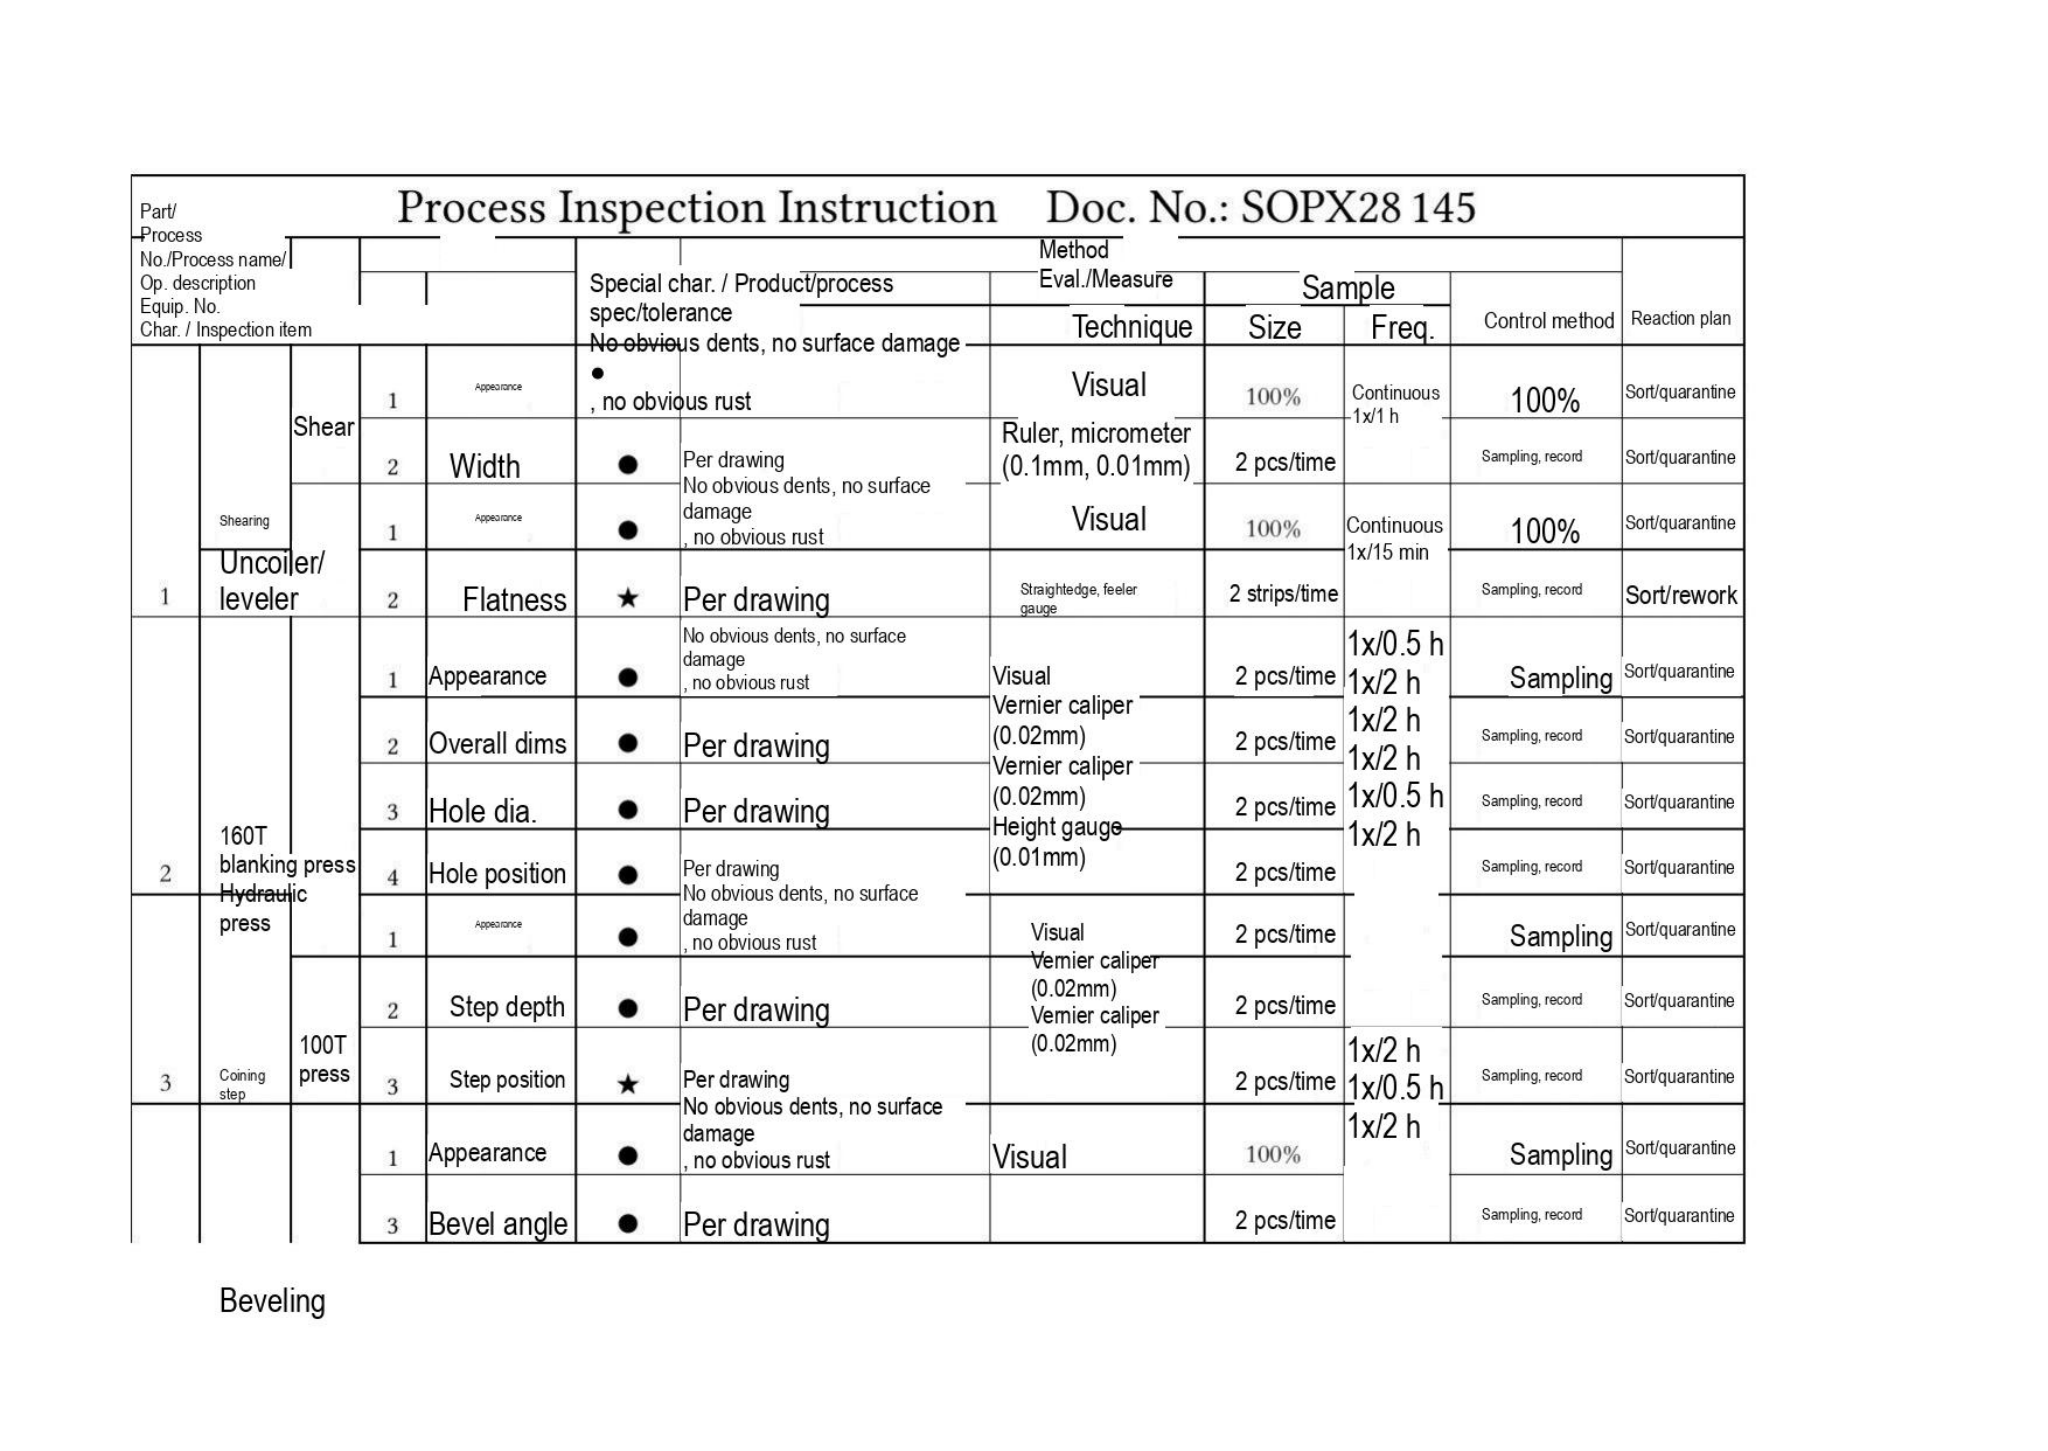# Process Inspection Instruction  Doc. No.: SOPX28 145

| Part/ Process No./Process name/ Op. description | | Equip. No. | Char. / Inspection item | | Special char. / Product/process spec/tolerance | | Method Eval./Measure Technique | Sample Size | Sample Freq. | Control method | Reaction plan |
|---|---|---|---|---|---|---|---|---|---|---|---|
| 1 | Shearing | Shear | 1 | Appearance | ● | No obvious dents, no surface damage, no obvious rust | Visual | 100% | Continuous 1x/1 h | 100% | Sort/quarantine |
| | | | 2 | Width | ● | Per drawing | Ruler, micrometer (0.1mm, 0.01mm) | 2 pcs/time | | Sampling, record | Sort/quarantine |
| | Uncoiler/ leveler | | 1 | Appearance | ● | No obvious dents, no surface damage, no obvious rust | Visual | 100% | Continuous 1x/15 min | 100% | Sort/quarantine |
| | | | 2 | Flatness | ★ | Per drawing | Straightedge, feeler gauge | 2 strips/time | | Sampling, record | Sort/rework |
| 2 | 160T blanking press ~~Hydraulic~~ press | | 1 | Appearance | ● | No obvious dents, no surface damage, no obvious rust | Visual | 2 pcs/time | 1x/0.5 h | Sampling | Sort/quarantine |
| | | | 2 | Overall dims | ● | Per drawing | Vernier caliper (0.02mm) | 2 pcs/time | 1x/2 h | Sampling, record | Sort/quarantine |
| | | | 3 | Hole dia. | ● | Per drawing | Vernier caliper (0.02mm) | 2 pcs/time | 1x/2 h | Sampling, record | Sort/quarantine |
| | | | 4 | Hole position | ● | Per drawing | Height gauge (0.01mm) | 2 pcs/time | 1x/2 h | Sampling, record | Sort/quarantine |
| 3 | Coining step | 100T press | 1 | Appearance | ● | No obvious dents, no surface damage, no obvious rust | Visual | 2 pcs/time | 1x/0.5 h | Sampling | Sort/quarantine |
| | | | 2 | Step depth | ● | Per drawing | Vernier caliper (0.02mm) | 2 pcs/time | 1x/2 h | Sampling, record | Sort/quarantine |
| | | | 3 | Step position | ★ | Per drawing | Vernier caliper (0.02mm) | 2 pcs/time | 1x/2 h | Sampling, record | Sort/quarantine |
| | | | 1 | Appearance | ● | No obvious dents, no surface damage, no obvious rust | Visual | 100% | 1x/0.5 h | Sampling | Sort/quarantine |
| | | | 3 | Bevel angle | ● | Per drawing | | 2 pcs/time | 1x/2 h | Sampling, record | Sort/quarantine |

Beveling
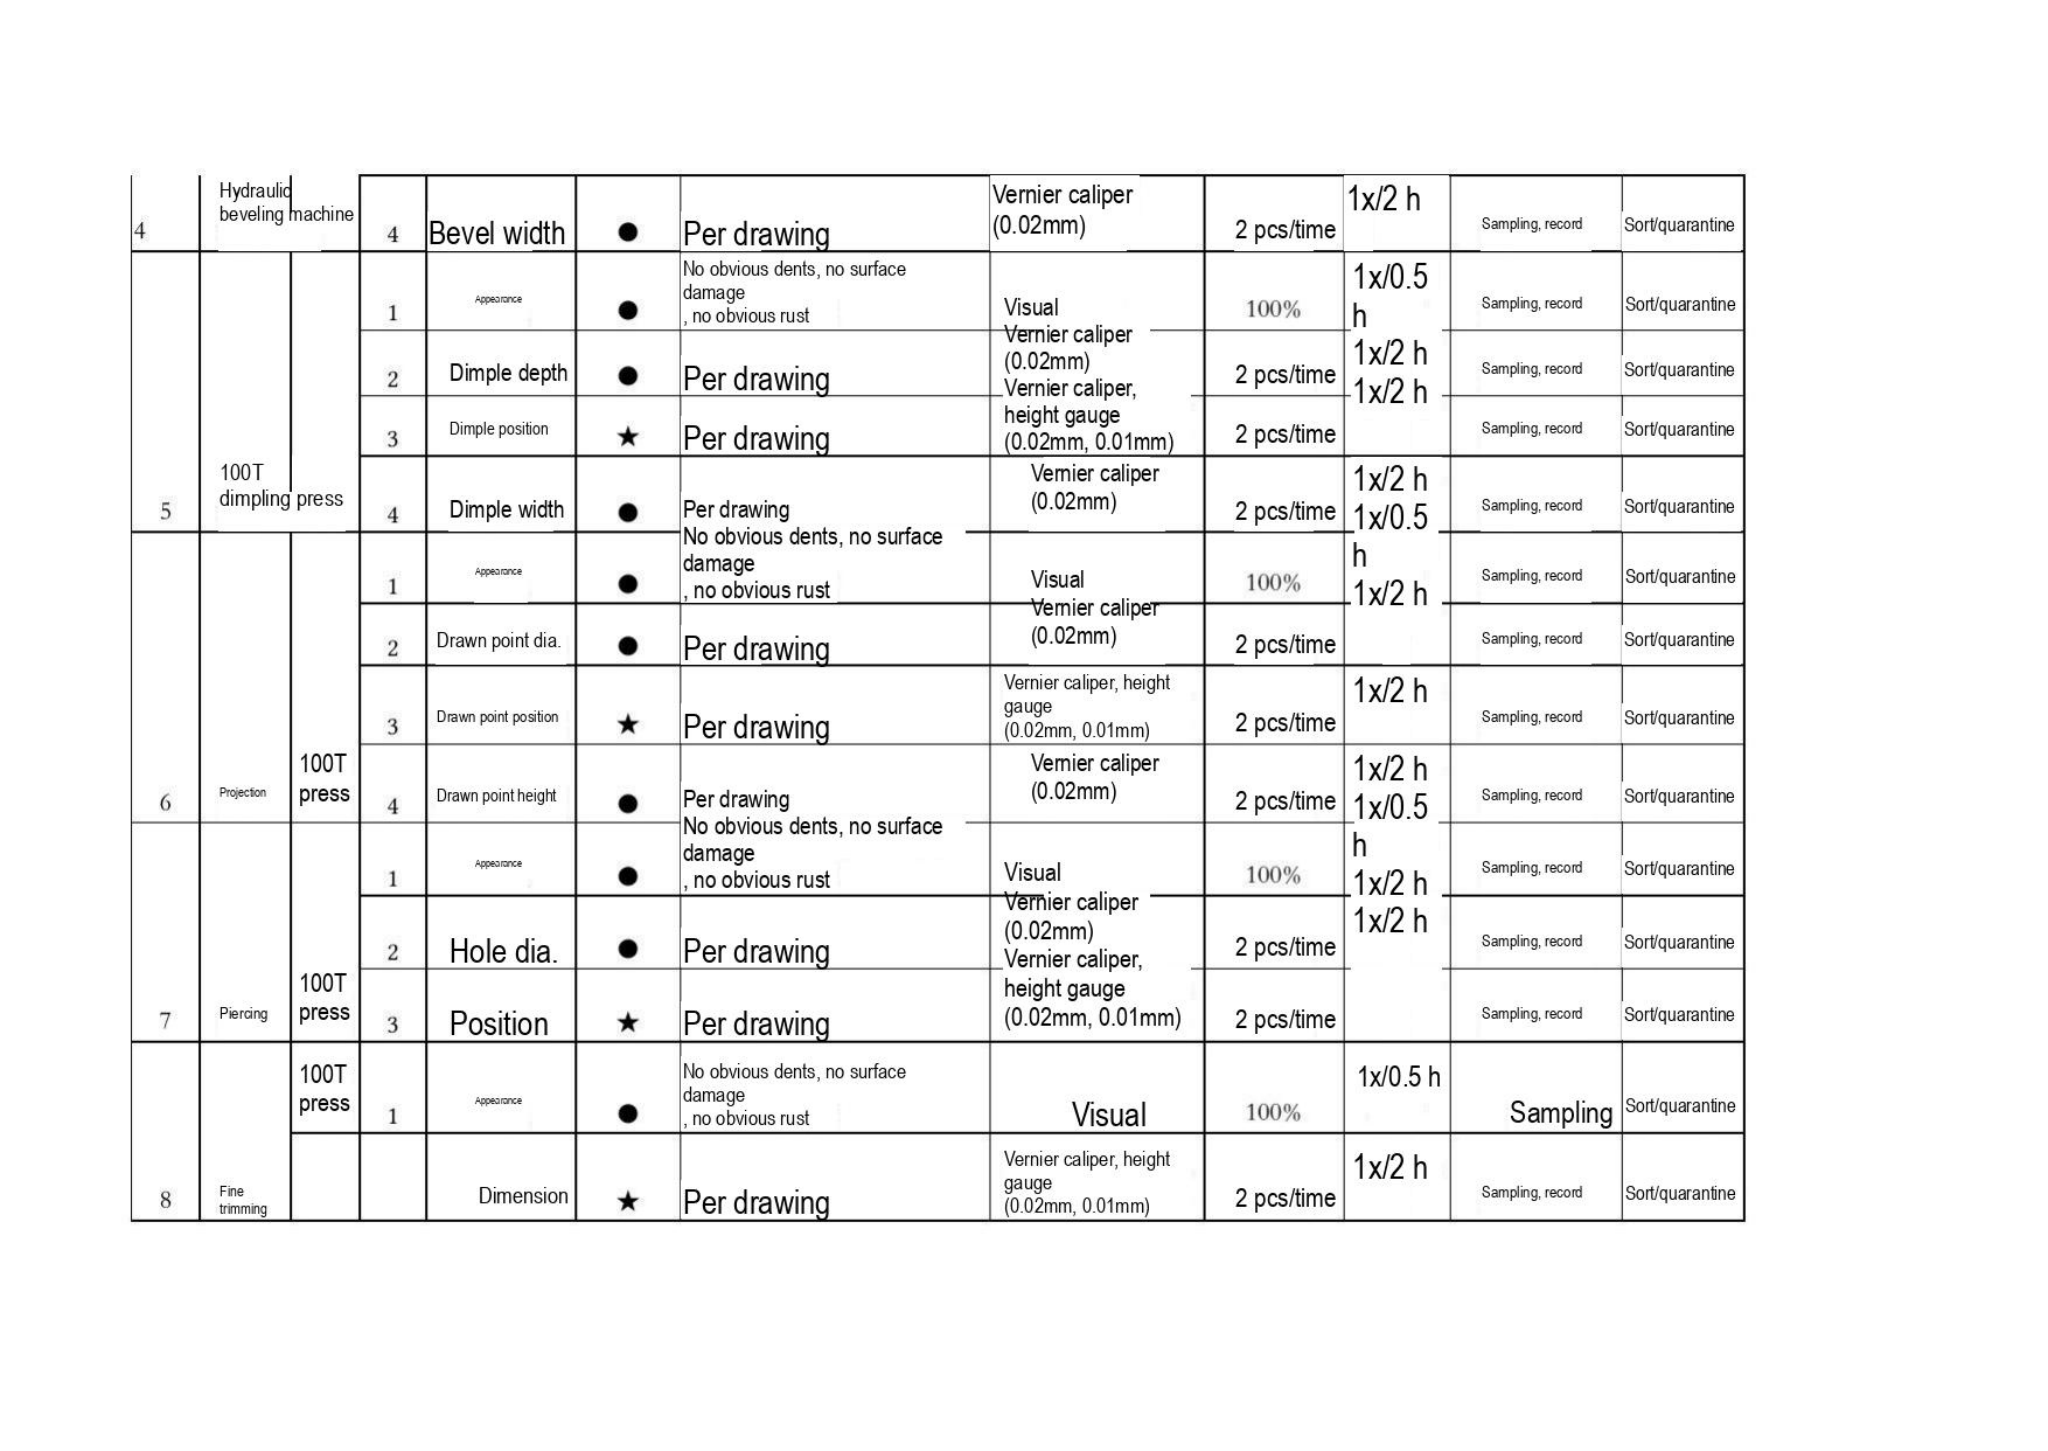| | | | | | | | | | | |
|---|---|---|---|---|---|---|---|---|---|---|
| 4 | Hydraulic beveling machine | | 4 | Bevel width | ● | Per drawing | Vernier caliper (0.02mm) | 2 pcs/time | 1x/2 h | Sampling, record | Sort/quarantine |
| 5 | 100T dimpling press | | 1 | Appearance | ● | No obvious dents, no surface damage , no obvious rust | Visual | 100% | 1x/0.5 h | Sampling, record | Sort/quarantine |
| | | | 2 | Dimple depth | ● | Per drawing | Vernier caliper (0.02mm) | 2 pcs/time | 1x/2 h | Sampling, record | Sort/quarantine |
| | | | 3 | Dimple position | ★ | Per drawing | Vernier caliper, height gauge (0.02mm, 0.01mm) | 2 pcs/time | 1x/2 h | Sampling, record | Sort/quarantine |
| | | | 4 | Dimple width | ● | Per drawing | Vernier caliper (0.02mm) | 2 pcs/time | 1x/2 h | Sampling, record | Sort/quarantine |
| 6 | Projection | 100T press | 1 | Appearance | ● | No obvious dents, no surface damage , no obvious rust | Visual | 100% | 1x/0.5 h | Sampling, record | Sort/quarantine |
| | | | 2 | Drawn point dia. | ● | Per drawing | Vernier caliper (0.02mm) | 2 pcs/time | 1x/2 h | Sampling, record | Sort/quarantine |
| | | | 3 | Drawn point position | ★ | Per drawing | Vernier caliper, height gauge (0.02mm, 0.01mm) | 2 pcs/time | 1x/2 h | Sampling, record | Sort/quarantine |
| | | | 4 | Drawn point height | ● | Per drawing | Vernier caliper (0.02mm) | 2 pcs/time | 1x/2 h | Sampling, record | Sort/quarantine |
| 7 | Piercing | 100T press | 1 | Appearance | ● | No obvious dents, no surface damage , no obvious rust | Visual | 100% | 1x/0.5 h | Sampling, record | Sort/quarantine |
| | | | 2 | Hole dia. | ● | Per drawing | Vernier caliper (0.02mm) | 2 pcs/time | 1x/2 h | Sampling, record | Sort/quarantine |
| | | | 3 | Position | ★ | Per drawing | Vernier caliper, height gauge (0.02mm, 0.01mm) | 2 pcs/time | 1x/2 h | Sampling, record | Sort/quarantine |
| 8 | Fine trimming | 100T press | 1 | Appearance | ● | No obvious dents, no surface damage , no obvious rust | Visual | 100% | 1x/0.5 h | Sampling | Sort/quarantine |
| | | | | Dimension | ★ | Per drawing | Vernier caliper, height gauge (0.02mm, 0.01mm) | 2 pcs/time | 1x/2 h | Sampling, record | Sort/quarantine |
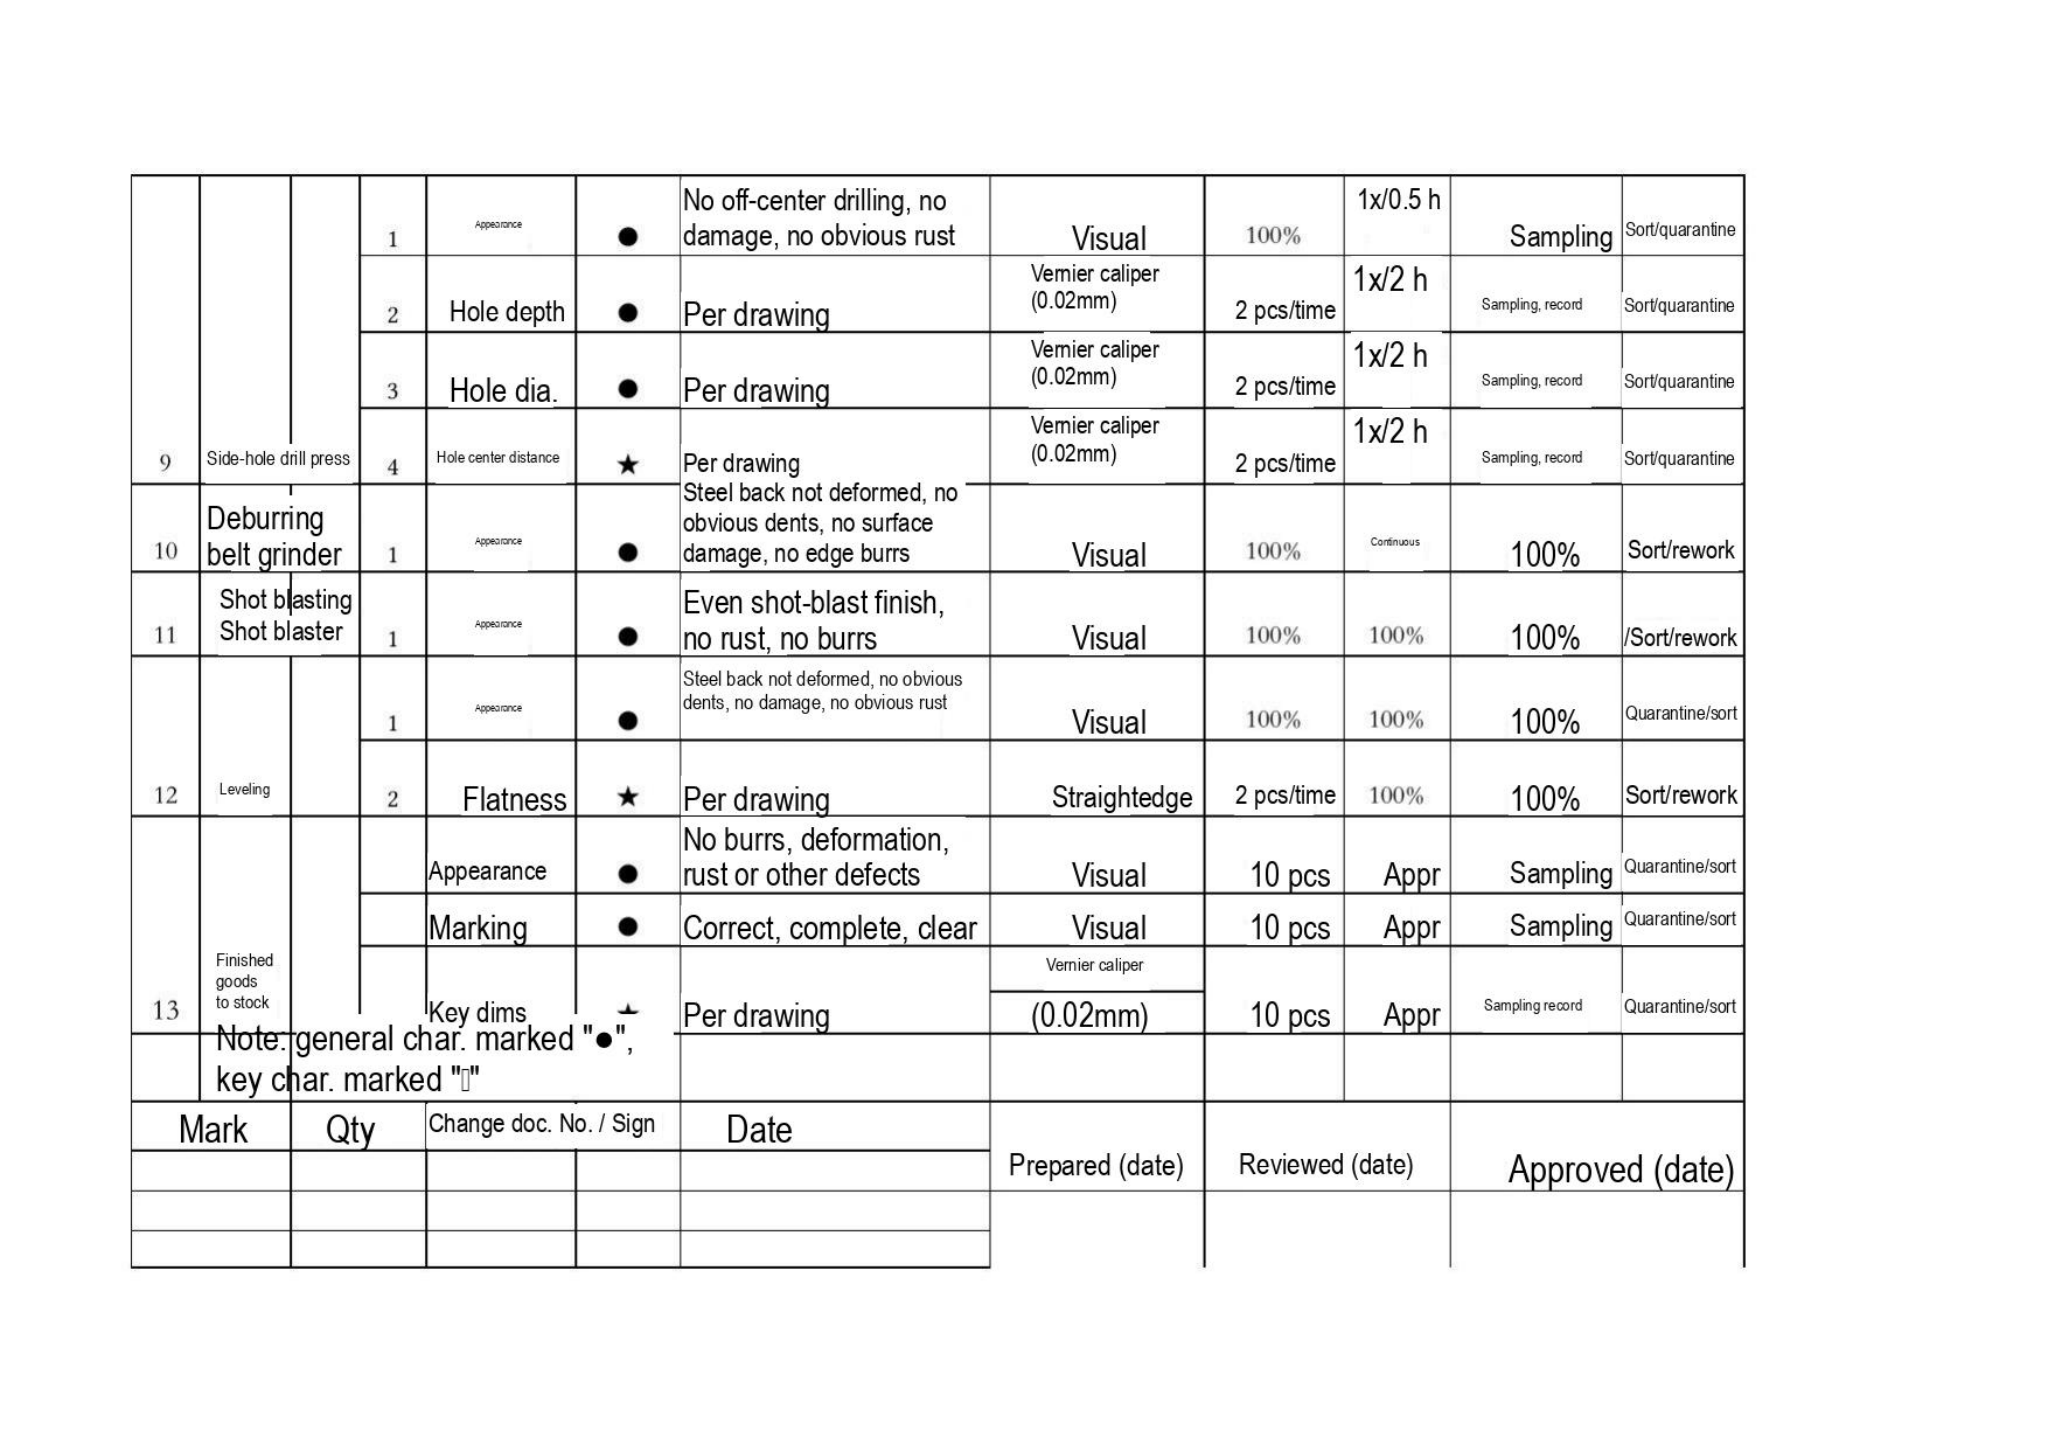|  |  |  |  |  |  |  |  |  |  |  |
|---|---|---|---|---|---|---|---|---|---|---|
|  |  | 1 | Appearance | ● | No off-center drilling, no damage, no obvious rust | Visual | 100% | 1x/0.5 h | Sampling | Sort/quarantine |
|  |  | 2 | Hole depth | ● | Per drawing | Vernier caliper (0.02mm) | 2 pcs/time | 1x/2 h | Sampling, record | Sort/quarantine |
|  |  | 3 | Hole dia. | ● | Per drawing | Vernier caliper (0.02mm) | 2 pcs/time | 1x/2 h | Sampling, record | Sort/quarantine |
| 9 | Side-hole drill press | 4 | Hole center distance | ★ | Per drawing | Vernier caliper (0.02mm) | 2 pcs/time | 1x/2 h | Sampling, record | Sort/quarantine |
| 10 | Deburring belt grinder | 1 | Appearance | ● | Steel back not deformed, no obvious dents, no surface damage, no edge burrs | Visual | 100% | Continuous | 100% | Sort/rework |
| 11 | Shot blasting Shot blaster | 1 | Appearance | ● | Even shot-blast finish, no rust, no burrs | Visual | 100% | 100% | 100% | /Sort/rework |
|  |  | 1 | Appearance | ● | Steel back not deformed, no obvious dents, no damage, no obvious rust | Visual | 100% | 100% | 100% | Quarantine/sort |
| 12 | Leveling | 2 | Flatness | ★ | Per drawing | Straightedge | 2 pcs/time | 100% | 100% | Sort/rework |
|  |  |  | Appearance | ● | No burrs, deformation, rust or other defects | Visual | 10 pcs | Appr | Sampling | Quarantine/sort |
|  |  |  | Marking | ● | Correct, complete, clear | Visual | 10 pcs | Appr | Sampling | Quarantine/sort |
| 13 | Finished goods to stock |  | Key dims |  | Per drawing | Vernier caliper (0.02mm) | 10 pcs | Appr | Sampling record | Quarantine/sort |
|  | Note: general char. marked "●", key char. marked "" |  |  |  |  |  |  |  |  |  |

| Mark | Qty | Change doc. No. / Sign |  | Date | Prepared (date) | Reviewed (date) | Approved (date) |
|---|---|---|---|---|---|---|---|
|  |  |  |  |  |  |  |  |
|  |  |  |  |  |  |  |  |
|  |  |  |  |  |  |  |  |